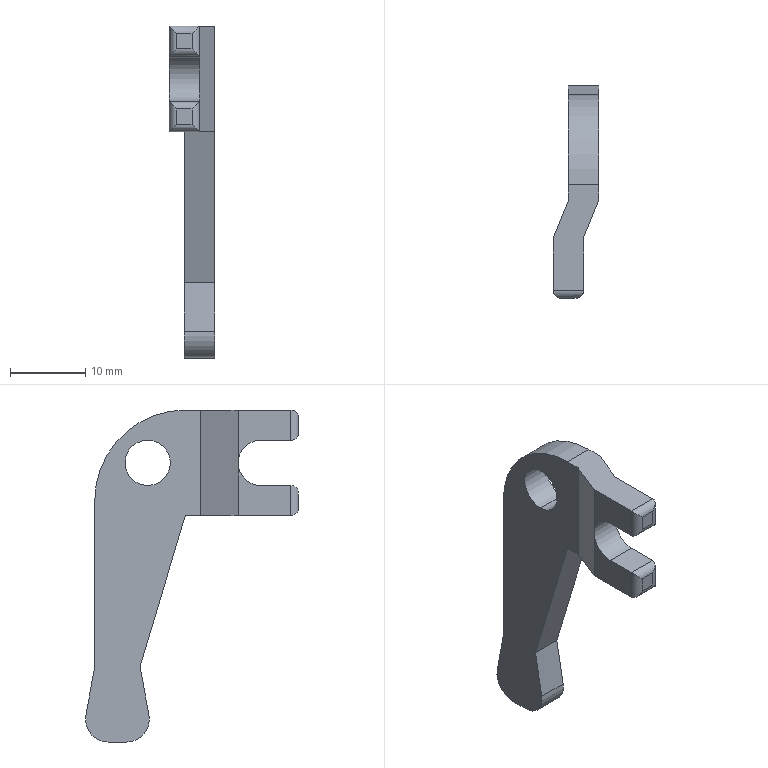Part | STEP file | 1 solid | 33 faces | box 6 x 28.229 x 44 mm | volume 2102 mm3 | plane 19 | cylinder 14 | commonest cylinder face diameters 2 x8 6 x5 24 x1